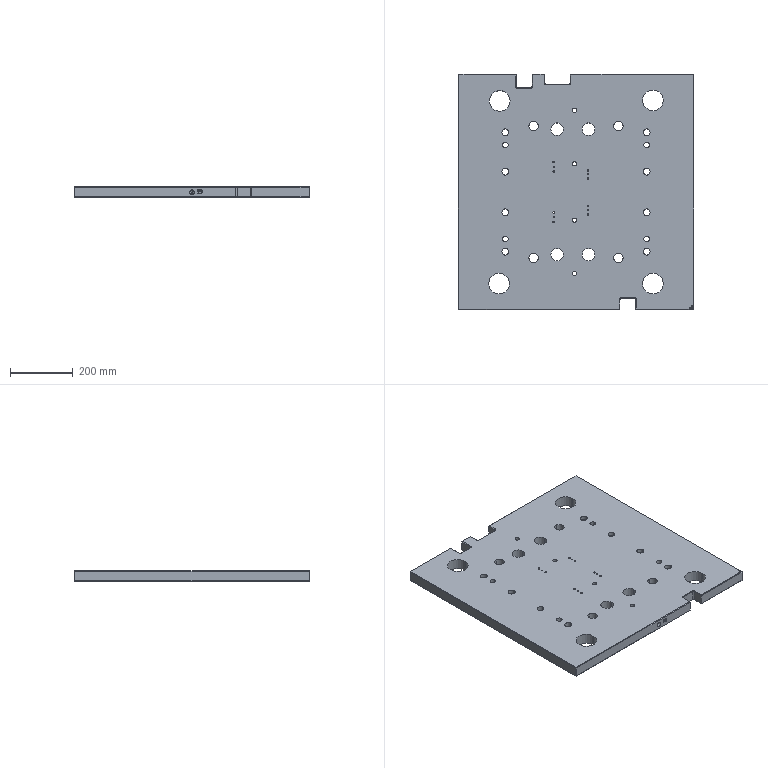Part | Creo | 1 solid | 670 faces | box 750 x 750 x 35 mm | volume 18292744 mm3 | cylinder 270 | plane 235 | other 101 | cone 64 | commonest cylinder face diameters 6 x62 5 x60 11 x16 22 x16 32 x16 3.8 x8